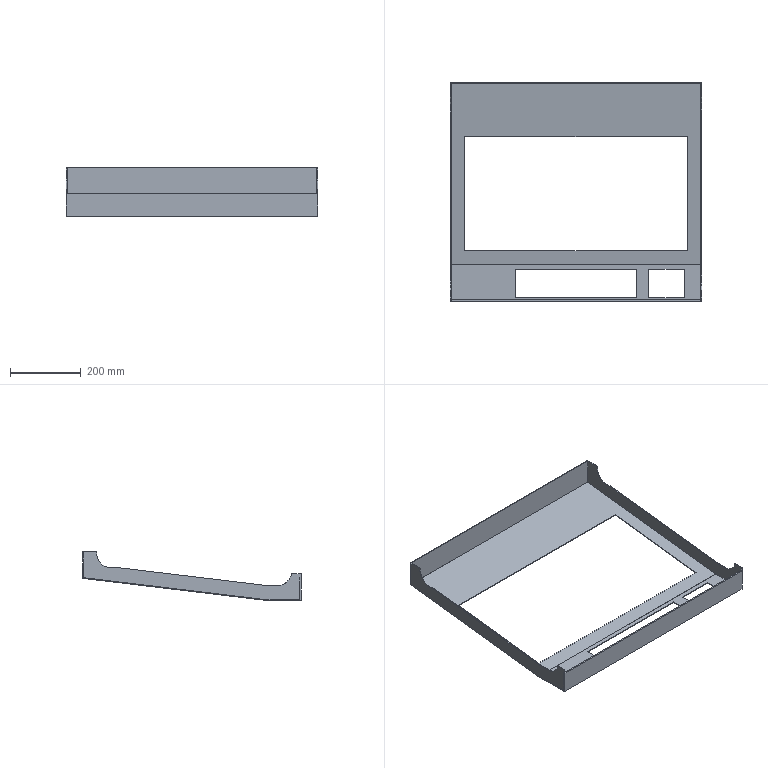Part | SolidWorks | features ICE 5, Cut 1, Extrusion 1 | 1 solid | 38 faces | box 710 x 618 x 137 mm | volume 789062 mm3 | plane 32 | cylinder 6 | commonest cylinder face diameters 80 x6
STEP:
#1=CARTESIAN_POINT('',(-708.,-79.693,30.051));
#2=VERTEX_POINT('',#1);
#3=CARTESIAN_POINT('',(-708.,-40.,75.));
#4=VERTEX_POINT('',#3);
#5=CARTESIAN_POINT('',(-708.,-79.693,70.051));
#6=DIRECTION('',(1.,0.,0.));
#7=DIRECTION('',(0.,0.,1.));
#8=AXIS2_PLACEMENT_3D('',#5,#6,#7);
#9=CIRCLE('',#8,40.);
#10=EDGE_CURVE('',#2,#4,#9,.T.);
#11=ORIENTED_EDGE('',*,*,#10,.F.);
#12=CARTESIAN_POINT('',(-706.,-79.693,30.051));
#13=VERTEX_POINT('',#12);
#14=CARTESIAN_POINT('',(-708.,-79.693,30.051));
#15=DIRECTION('',(1.,0.,0.));
#16=VECTOR('',#15,1000.);
#17=LINE('',#14,#16);
#18=EDGE_CURVE('',#2,#13,#17,.T.);
#19=ORIENTED_EDGE('',*,*,#18,.T.);
#20=CARTESIAN_POINT('',(-706.,-40.,75.));
#21=VERTEX_POINT('',#20);
#22=CARTESIAN_POINT('',(-706.,-79.693,70.051));
#23=DIRECTION('',(1.,0.,0.));
#24=DIRECTION('',(0.,0.,1.));
#25=AXIS2_PLACEMENT_3D('',#22,#23,#24);
#26=CIRCLE('',#25,40.);
#27=EDGE_CURVE('',#13,#21,#26,.T.);
#28=ORIENTED_EDGE('',*,*,#27,.T.);
#29=CARTESIAN_POINT('',(-708.,-40.,75.));
#30=DIRECTION('',(1.,0.,0.));
#31=VECTOR('',#30,1000.);
#32=LINE('',#29,#31);
#33=EDGE_CURVE('',#4,#21,#32,.T.);
#34=ORIENTED_EDGE('',*,*,#33,.F.);
#35=EDGE_LOOP('',(#11,#19,#28,#34));
#36=FACE_OUTER_BOUND('',#35,.T.);
#37=CARTESIAN_POINT('',(-708.,-79.693,70.051));
#38=DIRECTION('',(1.,0.,0.));
#39=DIRECTION('',(0.,0.,-1.));
#40=AXIS2_PLACEMENT_3D('',#37,#38,#39);
#41=CYLINDRICAL_SURFACE('',#40,40.);
#42=ADVANCED_FACE('',(#36),#41,.F.);
#43=CARTESIAN_POINT('',(-708.,-551.363,-20.439));
#44=VERTEX_POINT('',#43);
#45=CARTESIAN_POINT('',(-708.,-543.692,-19.697));
#46=VERTEX_POINT('',#45);
#47=CARTESIAN_POINT('',(-708.,-551.363,19.561));
#48=DIRECTION('',(1.,0.,0.));
#49=DIRECTION('',(0.,0.,1.));
#50=AXIS2_PLACEMENT_3D('',#47,#48,#49);
#51=CIRCLE('',#50,40.);
#52=EDGE_CURVE('',#44,#46,#51,.T.);
#53=ORIENTED_EDGE('',*,*,#52,.F.);
#54=CARTESIAN_POINT('',(-706.,-551.363,-20.439));
#55=VERTEX_POINT('',#54);
#56=CARTESIAN_POINT('',(-708.,-551.363,-20.439));
#57=DIRECTION('',(1.,0.,0.));
#58=VECTOR('',#57,1000.);
#59=LINE('',#56,#58);
#60=EDGE_CURVE('',#44,#55,#59,.T.);
#61=ORIENTED_EDGE('',*,*,#60,.T.);
#62=CARTESIAN_POINT('',(-706.,-543.692,-19.697));
#63=VERTEX_POINT('',#62);
#64=CARTESIAN_POINT('',(-706.,-551.363,19.561));
#65=DIRECTION('',(1.,0.,0.));
#66=DIRECTION('',(0.,0.,1.));
#67=AXIS2_PLACEMENT_3D('',#64,#65,#66);
#68=CIRCLE('',#67,40.);
#69=EDGE_CURVE('',#55,#63,#68,.T.);
#70=ORIENTED_EDGE('',*,*,#69,.T.);
#71=CARTESIAN_POINT('',(-708.,-543.692,-19.697));
#72=DIRECTION('',(1.,0.,0.));
#73=VECTOR('',#72,1000.);
#74=LINE('',#71,#73);
#75=EDGE_CURVE('',#46,#63,#74,.T.);
#76=ORIENTED_EDGE('',*,*,#75,.F.);
#77=EDGE_LOOP('',(#53,#61,#70,#76));
#78=FACE_OUTER_BOUND('',#77,.T.);
#79=CARTESIAN_POINT('',(-708.,-551.363,19.561));
#80=DIRECTION('',(1.,0.,0.));
#81=DIRECTION('',(0.,0.,-1.));
#82=AXIS2_PLACEMENT_3D('',#79,#80,#81);
#83=CYLINDRICAL_SURFACE('',#82,40.);
#84=ADVANCED_FACE('',(#78),#83,.F.);
#85=CARTESIAN_POINT('',(0.,-614.,1.));
#86=VERTEX_POINT('',#85);
#87=CARTESIAN_POINT('',(0.,-614.,-60.));
#88=VERTEX_POINT('',#87);
#89=CARTESIAN_POINT('',(0.,-614.,1.));
#90=DIRECTION('',(0.,0.,-1.));
#91=VECTOR('',#90,1000.);
#92=LINE('',#89,#91);
#93=EDGE_CURVE('',#86,#88,#92,.T.);
#94=ORIENTED_EDGE('',*,*,#93,.F.);
#95=CARTESIAN_POINT('',(0.,-618.,1.));
#96=VERTEX_POINT('',#95);
#97=CARTESIAN_POINT('',(0.,-618.,1.));
#98=DIRECTION('',(0.,1.,0.));
#99=VECTOR('',#98,1000.);
#100=LINE('',#97,#99);
#101=EDGE_CURVE('',#96,#86,#100,.T.);
#102=ORIENTED_EDGE('',*,*,#101,.F.);
#103=CARTESIAN_POINT('',(0.,-618.,13.));
#104=VERTEX_POINT('',#103);
#105=CARTESIAN_POINT('',(0.,-618.,13.));
#106=DIRECTION('',(0.,0.,-1.));
#107=VECTOR('',#106,1000.);
#108=LINE('',#105,#107);
#109=EDGE_CURVE('',#104,#96,#108,.T.);
#110=ORIENTED_EDGE('',*,*,#109,.F.);
#111=CARTESIAN_POINT('',(0.,-590.821,13.));
#112=VERTEX_POINT('',#111);
#113=CARTESIAN_POINT('',(0.,-618.,13.));
#114=DIRECTION('',(0.,-1.,0.));
#115=VECTOR('',#114,1000.);
#116=LINE('',#113,#115);
#117=EDGE_CURVE('',#112,#104,#116,.T.);
#118=ORIENTED_EDGE('',*,*,#117,.F.);
#119=CARTESIAN_POINT('',(0.,-543.692,-19.697));
#120=VERTEX_POINT('',#119);
#121=CARTESIAN_POINT('',(0.,-551.363,19.561));
#122=DIRECTION('',(-1.,0.,0.));
#123=DIRECTION('',(0.,0.,-1.));
#124=AXIS2_PLACEMENT_3D('',#121,#122,#123);
#125=CIRCLE('',#124,40.);
#126=EDGE_CURVE('',#120,#112,#125,.T.);
#127=ORIENTED_EDGE('',*,*,#126,.F.);
#128=CARTESIAN_POINT('',(0.,-515.,-19.697));
#129=VERTEX_POINT('',#128);
#130=CARTESIAN_POINT('',(0.,-515.,-19.697));
#131=DIRECTION('',(0.,-1.,0.));
#132=VECTOR('',#131,1000.);
#133=LINE('',#130,#132);
#134=EDGE_CURVE('',#129,#120,#133,.T.);
#135=ORIENTED_EDGE('',*,*,#134,.F.);
#136=CARTESIAN_POINT('',(0.,-90.171,31.448));
#137=VERTEX_POINT('',#136);
#138=CARTESIAN_POINT('',(0.,-90.171,31.448));
#139=DIRECTION('',(0.,-0.9928,-0.1195));
#140=VECTOR('',#139,1000.);
#141=LINE('',#138,#140);
#142=EDGE_CURVE('',#137,#129,#141,.T.);
#143=ORIENTED_EDGE('',*,*,#142,.F.);
#144=CARTESIAN_POINT('',(0.,-40.,75.));
#145=VERTEX_POINT('',#144);
#146=CARTESIAN_POINT('',(0.,-79.693,70.051));
#147=DIRECTION('',(-1.,0.,0.));
#148=DIRECTION('',(0.,0.,-1.));
#149=AXIS2_PLACEMENT_3D('',#146,#147,#148);
#150=CIRCLE('',#149,40.);
#151=EDGE_CURVE('',#145,#137,#150,.T.);
#152=ORIENTED_EDGE('',*,*,#151,.F.);
#153=CARTESIAN_POINT('',(0.,-2.,75.));
#154=VERTEX_POINT('',#153);
#155=CARTESIAN_POINT('',(0.,0.,75.));
#156=DIRECTION('',(0.,-1.,0.));
#157=VECTOR('',#156,1000.);
#158=LINE('',#155,#157);
#159=EDGE_CURVE('',#154,#145,#158,.T.);
#160=ORIENTED_EDGE('',*,*,#159,.F.);
#161=CARTESIAN_POINT('',(0.,-2.,1.774));
#162=VERTEX_POINT('',#161);
#163=CARTESIAN_POINT('',(0.,-2.,1.774));
#164=DIRECTION('',(0.,0.,1.));
#165=VECTOR('',#164,1000.);
#166=LINE('',#163,#165);
#167=EDGE_CURVE('',#162,#154,#166,.T.);
#168=ORIENTED_EDGE('',*,*,#167,.F.);
#169=CARTESIAN_POINT('',(0.,-515.12,-60.));
#170=VERTEX_POINT('',#169);
#171=CARTESIAN_POINT('',(0.,-515.12,-60.));
#172=DIRECTION('',(0.,0.9928,0.1195));
#173=VECTOR('',#172,1000.);
#174=LINE('',#171,#173);
#175=EDGE_CURVE('',#170,#162,#174,.T.);
#176=ORIENTED_EDGE('',*,*,#175,.F.);
#177=CARTESIAN_POINT('',(0.,-616.,-60.));
#178=DIRECTION('',(0.,1.,0.));
#179=VECTOR('',#178,1000.);
#180=LINE('',#177,#179);
#181=EDGE_CURVE('',#88,#170,#180,.T.);
#182=ORIENTED_EDGE('',*,*,#181,.F.);
#183=EDGE_LOOP('',(#94,#102,#110,#118,#127,#135,#143,#152,#160,#168,#176,#182));
#184=FACE_OUTER_BOUND('',#183,.T.);
#185=CARTESIAN_POINT('',(0.,-79.693,70.051));
#186=DIRECTION('',(1.,0.,0.));
#187=DIRECTION('',(0.,0.,-1.));
#188=AXIS2_PLACEMENT_3D('',#185,#186,#187);
#189=PLANE('',#188);
#190=ADVANCED_FACE('',(#184),#189,.F.);
#191=CARTESIAN_POINT('',(-147.,-528.,-60.));
#192=VERTEX_POINT('',#191);
#193=CARTESIAN_POINT('',(-47.,-528.,-60.));
#194=VERTEX_POINT('',#193);
#195=CARTESIAN_POINT('',(-147.,-528.,-60.));
#196=DIRECTION('',(1.,0.,0.));
#197=VECTOR('',#196,1000.);
#198=LINE('',#195,#197);
#199=EDGE_CURVE('',#192,#194,#198,.T.);
#200=ORIENTED_EDGE('',*,*,#199,.T.);
#201=CARTESIAN_POINT('',(-47.,-608.,-60.));
#202=VERTEX_POINT('',#201);
#203=CARTESIAN_POINT('',(-47.,-528.,-60.));
#204=DIRECTION('',(0.,-1.,0.));
#205=VECTOR('',#204,1000.);
#206=LINE('',#203,#205);
#207=EDGE_CURVE('',#194,#202,#206,.T.);
#208=ORIENTED_EDGE('',*,*,#207,.T.);
#209=CARTESIAN_POINT('',(-147.,-608.,-60.));
#210=VERTEX_POINT('',#209);
#211=CARTESIAN_POINT('',(-47.,-608.,-60.));
#212=DIRECTION('',(-1.,0.,0.));
#213=VECTOR('',#212,1000.);
#214=LINE('',#211,#213);
#215=EDGE_CURVE('',#202,#210,#214,.T.);
#216=ORIENTED_EDGE('',*,*,#215,.T.);
#217=CARTESIAN_POINT('',(-147.,-608.,-60.));
#218=DIRECTION('',(0.,1.,0.));
#219=VECTOR('',#218,1000.);
#220=LINE('',#217,#219);
#221=EDGE_CURVE('',#210,#192,#220,.T.);
#222=ORIENTED_EDGE('',*,*,#221,.T.);
#223=EDGE_LOOP('',(#200,#208,#216,#222));
#224=FACE_BOUND('',#223,.T.);
#225=CARTESIAN_POINT('',(-525.,-528.,-60.));
#226=VERTEX_POINT('',#225);
#227=CARTESIAN_POINT('',(-181.,-528.,-60.));
#228=VERTEX_POINT('',#227);
#229=CARTESIAN_POINT('',(-525.,-528.,-60.));
#230=DIRECTION('',(1.,0.,0.));
#231=VECTOR('',#230,1000.);
#232=LINE('',#229,#231);
#233=EDGE_CURVE('',#226,#228,#232,.T.);
#234=ORIENTED_EDGE('',*,*,#233,.T.);
#235=CARTESIAN_POINT('',(-181.,-608.,-60.));
#236=VERTEX_POINT('',#235);
#237=CARTESIAN_POINT('',(-181.,-528.,-60.));
#238=DIRECTION('',(0.,-1.,0.));
#239=VECTOR('',#238,1000.);
#240=LINE('',#237,#239);
#241=EDGE_CURVE('',#228,#236,#240,.T.);
#242=ORIENTED_EDGE('',*,*,#241,.T.);
#243=CARTESIAN_POINT('',(-525.,-608.,-60.));
#244=VERTEX_POINT('',#243);
#245=CARTESIAN_POINT('',(-181.,-608.,-60.));
#246=DIRECTION('',(-1.,0.,0.));
#247=VECTOR('',#246,1000.);
#248=LINE('',#245,#247);
#249=EDGE_CURVE('',#236,#244,#248,.T.);
#250=ORIENTED_EDGE('',*,*,#249,.T.);
#251=CARTESIAN_POINT('',(-525.,-608.,-60.));
#252=DIRECTION('',(0.,1.,0.));
#253=VECTOR('',#252,1000.);
#254=LINE('',#251,#253);
#255=EDGE_CURVE('',#244,#226,#254,.T.);
#256=ORIENTED_EDGE('',*,*,#255,.T.);
#257=EDGE_LOOP('',(#234,#242,#250,#256));
#258=FACE_BOUND('',#257,.T.);
#259=CARTESIAN_POINT('',(-706.,-614.,-60.));
#260=VERTEX_POINT('',#259);
#261=CARTESIAN_POINT('',(-706.,-614.,-60.));
#262=DIRECTION('',(-1.,0.,0.));
#263=VECTOR('',#262,1000.);
#264=LINE('',#261,#263);
#265=EDGE_CURVE('',#88,#260,#264,.T.);
#266=ORIENTED_EDGE('',*,*,#265,.F.);
#267=ORIENTED_EDGE('',*,*,#181,.T.);
#268=CARTESIAN_POINT('',(-706.,-515.12,-60.));
#269=VERTEX_POINT('',#268);
#270=CARTESIAN_POINT('',(-706.,-515.12,-60.));
#271=DIRECTION('',(1.,0.,0.));
#272=VECTOR('',#271,1000.);
#273=LINE('',#270,#272);
#274=EDGE_CURVE('',#269,#170,#273,.T.);
#275=ORIENTED_EDGE('',*,*,#274,.F.);
#276=CARTESIAN_POINT('',(-706.,-616.,-60.));
#277=DIRECTION('',(0.,1.,0.));
#278=VECTOR('',#277,1000.);
#279=LINE('',#276,#278);
#280=EDGE_CURVE('',#260,#269,#279,.T.);
#281=ORIENTED_EDGE('',*,*,#280,.F.);
#282=EDGE_LOOP('',(#266,#267,#275,#281));
#283=FACE_OUTER_BOUND('',#282,.T.);
#284=CARTESIAN_POINT('',(-706.,-616.,-60.));
#285=DIRECTION('',(0.,0.,-1.));
#286=DIRECTION('',(-1.,0.,0.));
#287=AXIS2_PLACEMENT_3D('',#284,#285,#286);
#288=PLANE('',#287);
#289=ADVANCED_FACE('',(#224,#258,#283),#288,.F.);
#290=CARTESIAN_POINT('',(-706.,-614.,1.));
#291=VERTEX_POINT('',#290);
#292=CARTESIAN_POINT('',(-706.,-614.,1.));
#293=DIRECTION('',(0.,0.,-1.));
#294=VECTOR('',#293,1000.);
#295=LINE('',#292,#294);
#296=EDGE_CURVE('',#291,#260,#295,.T.);
#297=ORIENTED_EDGE('',*,*,#296,.T.);
#298=ORIENTED_EDGE('',*,*,#280,.T.);
#299=CARTESIAN_POINT('',(-706.,-2.,1.774));
#300=VERTEX_POINT('',#299);
#301=CARTESIAN_POINT('',(-706.,-515.12,-60.));
#302=DIRECTION('',(0.,0.9928,0.1195));
#303=VECTOR('',#302,1000.);
#304=LINE('',#301,#303);
#305=EDGE_CURVE('',#269,#300,#304,.T.);
#306=ORIENTED_EDGE('',*,*,#305,.T.);
#307=CARTESIAN_POINT('',(-706.,-2.,75.));
#308=VERTEX_POINT('',#307);
#309=CARTESIAN_POINT('',(-706.,-2.,1.774));
#310=DIRECTION('',(0.,0.,1.));
#311=VECTOR('',#310,1000.);
#312=LINE('',#309,#311);
#313=EDGE_CURVE('',#300,#308,#312,.T.);
#314=ORIENTED_EDGE('',*,*,#313,.T.);
#315=CARTESIAN_POINT('',(-706.,-40.,75.));
#316=DIRECTION('',(0.,1.,0.));
#317=VECTOR('',#316,1000.);
#318=LINE('',#315,#317);
#319=EDGE_CURVE('',#21,#308,#318,.T.);
#320=ORIENTED_EDGE('',*,*,#319,.F.);
#321=ORIENTED_EDGE('',*,*,#27,.F.);
#322=CARTESIAN_POINT('',(-706.,-90.171,31.448));
#323=VERTEX_POINT('',#322);
#324=CARTESIAN_POINT('',(-706.,-79.693,70.051));
#325=DIRECTION('',(1.,0.,0.));
#326=DIRECTION('',(0.,0.,1.));
#327=AXIS2_PLACEMENT_3D('',#324,#325,#326);
#328=CIRCLE('',#327,40.);
#329=EDGE_CURVE('',#323,#13,#328,.T.);
#330=ORIENTED_EDGE('',*,*,#329,.F.);
#331=CARTESIAN_POINT('',(-706.,-515.,-19.697));
#332=VERTEX_POINT('',#331);
#333=CARTESIAN_POINT('',(-706.,-515.,-19.697));
#334=DIRECTION('',(0.,0.9928,0.1195));
#335=VECTOR('',#334,1000.);
#336=LINE('',#333,#335);
#337=EDGE_CURVE('',#332,#323,#336,.T.);
#338=ORIENTED_EDGE('',*,*,#337,.F.);
#339=CARTESIAN_POINT('',(-706.,-543.692,-19.697));
#340=DIRECTION('',(0.,1.,0.));
#341=VECTOR('',#340,1000.);
#342=LINE('',#339,#341);
#343=EDGE_CURVE('',#63,#332,#342,.T.);
#344=ORIENTED_EDGE('',*,*,#343,.F.);
#345=ORIENTED_EDGE('',*,*,#69,.F.);
#346=CARTESIAN_POINT('',(-706.,-590.821,13.));
#347=VERTEX_POINT('',#346);
#348=CARTESIAN_POINT('',(-706.,-551.363,19.561));
#349=DIRECTION('',(1.,0.,0.));
#350=DIRECTION('',(0.,0.,1.));
#351=AXIS2_PLACEMENT_3D('',#348,#349,#350);
#352=CIRCLE('',#351,40.);
#353=EDGE_CURVE('',#347,#55,#352,.T.);
#354=ORIENTED_EDGE('',*,*,#353,.F.);
#355=CARTESIAN_POINT('',(-706.,-618.,13.));
#356=VERTEX_POINT('',#355);
#357=CARTESIAN_POINT('',(-706.,-618.,13.));
#358=DIRECTION('',(0.,1.,0.));
#359=VECTOR('',#358,1000.);
#360=LINE('',#357,#359);
#361=EDGE_CURVE('',#356,#347,#360,.T.);
#362=ORIENTED_EDGE('',*,*,#361,.F.);
#363=CARTESIAN_POINT('',(-706.,-618.,1.));
#364=VERTEX_POINT('',#363);
#365=CARTESIAN_POINT('',(-706.,-618.,-62.));
#366=DIRECTION('',(0.,0.,1.));
#367=VECTOR('',#366,1000.);
#368=LINE('',#365,#367);
#369=EDGE_CURVE('',#364,#356,#368,.T.);
#370=ORIENTED_EDGE('',*,*,#369,.F.);
#371=CARTESIAN_POINT('',(-706.,-618.,1.));
#372=DIRECTION('',(0.,-1.,0.));
#373=VECTOR('',#372,1000.);
#374=LINE('',#371,#373);
#375=EDGE_CURVE('',#291,#364,#374,.T.);
#376=ORIENTED_EDGE('',*,*,#375,.F.);
#377=EDGE_LOOP('',(#297,#298,#306,#314,#320,#321,#330,#338,#344,#345,#354,#362,#370,#376));
#378=FACE_OUTER_BOUND('',#377,.T.);
#379=CARTESIAN_POINT('',(-706.,-551.363,19.561));
#380=DIRECTION('',(-1.,0.,0.));
#381=DIRECTION('',(0.,0.,1.));
#382=AXIS2_PLACEMENT_3D('',#379,#380,#381);
#383=PLANE('',#382);
#384=ADVANCED_FACE('',(#378),#383,.F.);
#385=CARTESIAN_POINT('',(-667.,-152.,-18.299));
#386=VERTEX_POINT('',#385);
#387=CARTESIAN_POINT('',(-39.,-152.,-18.299));
#388=VERTEX_POINT('',#387);
#389=CARTESIAN_POINT('',(-39.,-152.,-18.299));
#390=DIRECTION('',(1.,0.,0.));
#391=VECTOR('',#390,1000.);
#392=LINE('',#389,#391);
#393=EDGE_CURVE('',#386,#388,#392,.T.);
#394=ORIENTED_EDGE('',*,*,#393,.F.);
#395=CARTESIAN_POINT('',(-667.,-475.,-57.184));
#396=VERTEX_POINT('',#395);
#397=CARTESIAN_POINT('',(-667.,-140.928,-16.966));
#398=DIRECTION('',(0.,0.9928,0.1195));
#399=VECTOR('',#398,1000.);
#400=LINE('',#397,#399);
#401=EDGE_CURVE('',#396,#386,#400,.T.);
#402=ORIENTED_EDGE('',*,*,#401,.F.);
#403=CARTESIAN_POINT('',(-39.,-475.,-57.184));
#404=VERTEX_POINT('',#403);
#405=CARTESIAN_POINT('',(-39.,-475.,-57.184));
#406=DIRECTION('',(-1.,0.,0.));
#407=VECTOR('',#406,1000.);
#408=LINE('',#405,#407);
#409=EDGE_CURVE('',#404,#396,#408,.T.);
#410=ORIENTED_EDGE('',*,*,#409,.F.);
#411=CARTESIAN_POINT('',(-39.,-140.928,-16.966));
#412=DIRECTION('',(0.,-0.9928,-0.1195));
#413=VECTOR('',#412,1000.);
#414=LINE('',#411,#413);
#415=EDGE_CURVE('',#388,#404,#414,.T.);
#416=ORIENTED_EDGE('',*,*,#415,.F.);
#417=EDGE_LOOP('',(#394,#402,#410,#416));
#418=FACE_BOUND('',#417,.T.);
#419=CARTESIAN_POINT('',(2.,-515.,-62.));
#420=VERTEX_POINT('',#419);
#421=CARTESIAN_POINT('',(-708.,-515.,-62.));
#422=VERTEX_POINT('',#421);
#423=CARTESIAN_POINT('',(2.,-515.,-62.));
#424=DIRECTION('',(-1.,0.,0.));
#425=VECTOR('',#424,1000.);
#426=LINE('',#423,#425);
#427=EDGE_CURVE('',#420,#422,#426,.T.);
#428=ORIENTED_EDGE('',*,*,#427,.T.);
#429=CARTESIAN_POINT('',(-708.,0.,0.));
#430=VERTEX_POINT('',#429);
#431=CARTESIAN_POINT('',(-708.,0.,0.));
#432=DIRECTION('',(0.,-0.9928,-0.1195));
#433=VECTOR('',#432,1000.);
#434=LINE('',#431,#433);
#435=EDGE_CURVE('',#430,#422,#434,.T.);
#436=ORIENTED_EDGE('',*,*,#435,.F.);
#437=CARTESIAN_POINT('',(2.,0.,0.));
#438=VERTEX_POINT('',#437);
#439=CARTESIAN_POINT('',(2.,0.,0.));
#440=DIRECTION('',(-1.,0.,0.));
#441=VECTOR('',#440,1000.);
#442=LINE('',#439,#441);
#443=EDGE_CURVE('',#438,#430,#442,.T.);
#444=ORIENTED_EDGE('',*,*,#443,.F.);
#445=CARTESIAN_POINT('',(2.,-515.,-62.));
#446=DIRECTION('',(0.,0.9928,0.1195));
#447=VECTOR('',#446,1000.);
#448=LINE('',#445,#447);
#449=EDGE_CURVE('',#420,#438,#448,.T.);
#450=ORIENTED_EDGE('',*,*,#449,.F.);
#451=EDGE_LOOP('',(#428,#436,#444,#450));
#452=FACE_OUTER_BOUND('',#451,.T.);
#453=CARTESIAN_POINT('',(2.,-515.,-62.));
#454=DIRECTION('',(0.,-0.1195,0.9928));
#455=DIRECTION('',(0.,-0.9928,-0.1195));
#456=AXIS2_PLACEMENT_3D('',#453,#454,#455);
#457=PLANE('',#456);
#458=ADVANCED_FACE('',(#418,#452),#457,.F.);
#459=ORIENTED_EDGE('',*,*,#443,.T.);
#460=CARTESIAN_POINT('',(-708.,0.,75.));
#461=VERTEX_POINT('',#460);
#462=CARTESIAN_POINT('',(-708.,0.,75.));
#463=DIRECTION('',(0.,0.,-1.));
#464=VECTOR('',#463,1000.);
#465=LINE('',#462,#464);
#466=EDGE_CURVE('',#461,#430,#465,.T.);
#467=ORIENTED_EDGE('',*,*,#466,.F.);
#468=CARTESIAN_POINT('',(2.,0.,75.));
#469=VERTEX_POINT('',#468);
#470=CARTESIAN_POINT('',(2.,0.,75.));
#471=DIRECTION('',(-1.,0.,0.));
#472=VECTOR('',#471,1000.);
#473=LINE('',#470,#472);
#474=EDGE_CURVE('',#469,#461,#473,.T.);
#475=ORIENTED_EDGE('',*,*,#474,.F.);
#476=CARTESIAN_POINT('',(2.,0.,0.));
#477=DIRECTION('',(0.,0.,1.));
#478=VECTOR('',#477,1000.);
#479=LINE('',#476,#478);
#480=EDGE_CURVE('',#438,#469,#479,.T.);
#481=ORIENTED_EDGE('',*,*,#480,.F.);
#482=EDGE_LOOP('',(#459,#467,#475,#481));
#483=FACE_OUTER_BOUND('',#482,.T.);
#484=CARTESIAN_POINT('',(2.,0.,0.));
#485=DIRECTION('',(0.,-1.,0.));
#486=DIRECTION('',(0.,0.,-1.));
#487=AXIS2_PLACEMENT_3D('',#484,#485,#486);
#488=PLANE('',#487);
#489=ADVANCED_FACE('',(#483),#488,.F.);
#490=ORIENTED_EDGE('',*,*,#474,.T.);
#491=CARTESIAN_POINT('',(-708.,-40.,75.));
#492=DIRECTION('',(0.,1.,0.));
#493=VECTOR('',#492,1000.);
#494=LINE('',#491,#493);
#495=EDGE_CURVE('',#4,#461,#494,.T.);
#496=ORIENTED_EDGE('',*,*,#495,.F.);
#497=ORIENTED_EDGE('',*,*,#33,.T.);
#498=ORIENTED_EDGE('',*,*,#319,.T.);
#499=CARTESIAN_POINT('',(-706.,-2.,75.));
#500=DIRECTION('',(1.,0.,0.));
#501=VECTOR('',#500,1000.);
#502=LINE('',#499,#501);
#503=EDGE_CURVE('',#308,#154,#502,.T.);
#504=ORIENTED_EDGE('',*,*,#503,.T.);
#505=ORIENTED_EDGE('',*,*,#159,.T.);
#506=CARTESIAN_POINT('',(2.,-40.,75.));
#507=VERTEX_POINT('',#506);
#508=CARTESIAN_POINT('',(2.,-40.,75.));
#509=DIRECTION('',(-1.,0.,0.));
#510=VECTOR('',#509,1000.);
#511=LINE('',#508,#510);
#512=EDGE_CURVE('',#507,#145,#511,.T.);
#513=ORIENTED_EDGE('',*,*,#512,.F.);
#514=CARTESIAN_POINT('',(2.,0.,75.));
#515=DIRECTION('',(0.,-1.,0.));
#516=VECTOR('',#515,1000.);
#517=LINE('',#514,#516);
#518=EDGE_CURVE('',#469,#507,#517,.T.);
#519=ORIENTED_EDGE('',*,*,#518,.F.);
#520=EDGE_LOOP('',(#490,#496,#497,#498,#504,#505,#513,#519));
#521=FACE_OUTER_BOUND('',#520,.T.);
#522=CARTESIAN_POINT('',(2.,0.,75.));
#523=DIRECTION('',(0.,0.,-1.));
#524=DIRECTION('',(-1.,0.,0.));
#525=AXIS2_PLACEMENT_3D('',#522,#523,#524);
#526=PLANE('',#525);
#527=ADVANCED_FACE('',(#521),#526,.F.);
#528=ORIENTED_EDGE('',*,*,#151,.T.);
#529=CARTESIAN_POINT('',(2.,-90.171,31.448));
#530=VERTEX_POINT('',#529);
#531=CARTESIAN_POINT('',(2.,-90.171,31.448));
#532=DIRECTION('',(-1.,0.,0.));
#533=VECTOR('',#532,1000.);
#534=LINE('',#531,#533);
#535=EDGE_CURVE('',#530,#137,#534,.T.);
#536=ORIENTED_EDGE('',*,*,#535,.F.);
#537=CARTESIAN_POINT('',(2.,-79.693,70.051));
#538=DIRECTION('',(-1.,0.,0.));
#539=DIRECTION('',(0.,0.,-1.));
#540=AXIS2_PLACEMENT_3D('',#537,#538,#539);
#541=CIRCLE('',#540,40.);
#542=EDGE_CURVE('',#507,#530,#541,.T.);
#543=ORIENTED_EDGE('',*,*,#542,.F.);
#544=ORIENTED_EDGE('',*,*,#512,.T.);
#545=EDGE_LOOP('',(#528,#536,#543,#544));
#546=FACE_OUTER_BOUND('',#545,.T.);
#547=CARTESIAN_POINT('',(2.,-79.693,70.051));
#548=DIRECTION('',(-1.,0.,0.));
#549=DIRECTION('',(0.,0.,1.));
#550=AXIS2_PLACEMENT_3D('',#547,#548,#549);
#551=CYLINDRICAL_SURFACE('',#550,40.);
#552=ADVANCED_FACE('',(#546),#551,.F.);
#553=ORIENTED_EDGE('',*,*,#142,.T.);
#554=CARTESIAN_POINT('',(2.,-515.,-19.697));
#555=VERTEX_POINT('',#554);
#556=CARTESIAN_POINT('',(2.,-515.,-19.697));
#557=DIRECTION('',(-1.,0.,0.));
#558=VECTOR('',#557,1000.);
#559=LINE('',#556,#558);
#560=EDGE_CURVE('',#555,#129,#559,.T.);
#561=ORIENTED_EDGE('',*,*,#560,.F.);
#562=CARTESIAN_POINT('',(2.,-90.171,31.448));
#563=DIRECTION('',(0.,-0.9928,-0.1195));
#564=VECTOR('',#563,1000.);
#565=LINE('',#562,#564);
#566=EDGE_CURVE('',#530,#555,#565,.T.);
#567=ORIENTED_EDGE('',*,*,#566,.F.);
#568=ORIENTED_EDGE('',*,*,#535,.T.);
#569=EDGE_LOOP('',(#553,#561,#567,#568));
#570=FACE_OUTER_BOUND('',#569,.T.);
#571=CARTESIAN_POINT('',(2.,-90.171,31.448));
#572=DIRECTION('',(0.,0.1195,-0.9928));
#573=DIRECTION('',(0.,0.9928,0.1195));
#574=AXIS2_PLACEMENT_3D('',#571,#572,#573);
#575=PLANE('',#574);
#576=ADVANCED_FACE('',(#570),#575,.F.);
#577=ORIENTED_EDGE('',*,*,#134,.T.);
#578=CARTESIAN_POINT('',(2.,-543.692,-19.697));
#579=VERTEX_POINT('',#578);
#580=CARTESIAN_POINT('',(2.,-543.692,-19.697));
#581=DIRECTION('',(-1.,0.,0.));
#582=VECTOR('',#581,1000.);
#583=LINE('',#580,#582);
#584=EDGE_CURVE('',#579,#120,#583,.T.);
#585=ORIENTED_EDGE('',*,*,#584,.F.);
#586=CARTESIAN_POINT('',(2.,-515.,-19.697));
#587=DIRECTION('',(0.,-1.,0.));
#588=VECTOR('',#587,1000.);
#589=LINE('',#586,#588);
#590=EDGE_CURVE('',#555,#579,#589,.T.);
#591=ORIENTED_EDGE('',*,*,#590,.F.);
#592=ORIENTED_EDGE('',*,*,#560,.T.);
#593=EDGE_LOOP('',(#577,#585,#591,#592));
#594=FACE_OUTER_BOUND('',#593,.T.);
#595=CARTESIAN_POINT('',(2.,-515.,-19.697));
#596=DIRECTION('',(0.,0.,-1.));
#597=DIRECTION('',(-1.,0.,0.));
#598=AXIS2_PLACEMENT_3D('',#595,#596,#597);
#599=PLANE('',#598);
#600=ADVANCED_FACE('',(#594),#599,.F.);
#601=ORIENTED_EDGE('',*,*,#126,.T.);
#602=CARTESIAN_POINT('',(2.,-590.821,13.));
#603=VERTEX_POINT('',#602);
#604=CARTESIAN_POINT('',(2.,-590.821,13.));
#605=DIRECTION('',(-1.,0.,0.));
#606=VECTOR('',#605,1000.);
#607=LINE('',#604,#606);
#608=EDGE_CURVE('',#603,#112,#607,.T.);
#609=ORIENTED_EDGE('',*,*,#608,.F.);
#610=CARTESIAN_POINT('',(2.,-551.363,19.561));
#611=DIRECTION('',(-1.,0.,0.));
#612=DIRECTION('',(0.,0.,-1.));
#613=AXIS2_PLACEMENT_3D('',#610,#611,#612);
#614=CIRCLE('',#613,40.);
#615=EDGE_CURVE('',#579,#603,#614,.T.);
#616=ORIENTED_EDGE('',*,*,#615,.F.);
#617=ORIENTED_EDGE('',*,*,#584,.T.);
#618=EDGE_LOOP('',(#601,#609,#616,#617));
#619=FACE_OUTER_BOUND('',#618,.T.);
#620=CARTESIAN_POINT('',(2.,-551.363,19.561));
#621=DIRECTION('',(-1.,0.,0.));
#622=DIRECTION('',(0.,0.,1.));
#623=AXIS2_PLACEMENT_3D('',#620,#621,#622);
#624=CYLINDRICAL_SURFACE('',#623,40.);
#625=ADVANCED_FACE('',(#619),#624,.F.);
#626=ORIENTED_EDGE('',*,*,#117,.T.);
#627=CARTESIAN_POINT('',(2.,-618.,13.));
#628=VERTEX_POINT('',#627);
#629=CARTESIAN_POINT('',(2.,-618.,13.));
#630=DIRECTION('',(-1.,0.,0.));
#631=VECTOR('',#630,1000.);
#632=LINE('',#629,#631);
#633=EDGE_CURVE('',#628,#104,#632,.T.);
#634=ORIENTED_EDGE('',*,*,#633,.F.);
#635=CARTESIAN_POINT('',(2.,-618.,13.));
#636=DIRECTION('',(0.,-1.,0.));
#637=VECTOR('',#636,1000.);
#638=LINE('',#635,#637);
#639=EDGE_CURVE('',#603,#628,#638,.T.);
#640=ORIENTED_EDGE('',*,*,#639,.F.);
#641=ORIENTED_EDGE('',*,*,#608,.T.);
#642=EDGE_LOOP('',(#626,#634,#640,#641));
#643=FACE_OUTER_BOUND('',#642,.T.);
#644=CARTESIAN_POINT('',(2.,-618.,13.));
#645=DIRECTION('',(0.,0.,-1.));
#646=DIRECTION('',(-1.,0.,0.));
#647=AXIS2_PLACEMENT_3D('',#644,#645,#646);
#648=PLANE('',#647);
#649=ADVANCED_FACE('',(#643),#648,.F.);
#650=ORIENTED_EDGE('',*,*,#109,.T.);
#651=CARTESIAN_POINT('',(-706.,-618.,1.));
#652=DIRECTION('',(1.,0.,0.));
#653=VECTOR('',#652,1000.);
#654=LINE('',#651,#653);
#655=EDGE_CURVE('',#364,#96,#654,.T.);
#656=ORIENTED_EDGE('',*,*,#655,.F.);
#657=ORIENTED_EDGE('',*,*,#369,.T.);
#658=CARTESIAN_POINT('',(-708.,-618.,13.));
#659=VERTEX_POINT('',#658);
#660=CARTESIAN_POINT('',(-708.,-618.,13.));
#661=DIRECTION('',(1.,0.,0.));
#662=VECTOR('',#661,1000.);
#663=LINE('',#660,#662);
#664=EDGE_CURVE('',#659,#356,#663,.T.);
#665=ORIENTED_EDGE('',*,*,#664,.F.);
#666=CARTESIAN_POINT('',(-708.,-618.,-62.));
#667=VERTEX_POINT('',#666);
#668=CARTESIAN_POINT('',(-708.,-618.,-62.));
#669=DIRECTION('',(0.,0.,1.));
#670=VECTOR('',#669,1000.);
#671=LINE('',#668,#670);
#672=EDGE_CURVE('',#667,#659,#671,.T.);
#673=ORIENTED_EDGE('',*,*,#672,.F.);
#674=CARTESIAN_POINT('',(2.,-618.,-62.));
#675=VERTEX_POINT('',#674);
#676=CARTESIAN_POINT('',(2.,-618.,-62.));
#677=DIRECTION('',(-1.,0.,0.));
#678=VECTOR('',#677,1000.);
#679=LINE('',#676,#678);
#680=EDGE_CURVE('',#675,#667,#679,.T.);
#681=ORIENTED_EDGE('',*,*,#680,.F.);
#682=CARTESIAN_POINT('',(2.,-618.,13.));
#683=DIRECTION('',(0.,0.,-1.));
#684=VECTOR('',#683,1000.);
#685=LINE('',#682,#684);
#686=EDGE_CURVE('',#628,#675,#685,.T.);
#687=ORIENTED_EDGE('',*,*,#686,.F.);
#688=ORIENTED_EDGE('',*,*,#633,.T.);
#689=EDGE_LOOP('',(#650,#656,#657,#665,#673,#681,#687,#688));
#690=FACE_OUTER_BOUND('',#689,.T.);
#691=CARTESIAN_POINT('',(2.,-618.,13.));
#692=DIRECTION('',(0.,1.,0.));
#693=DIRECTION('',(0.,0.,1.));
#694=AXIS2_PLACEMENT_3D('',#691,#692,#693);
#695=PLANE('',#694);
#696=ADVANCED_FACE('',(#690),#695,.F.);
#697=CARTESIAN_POINT('',(-181.,-608.,-62.));
#698=VERTEX_POINT('',#697);
#699=CARTESIAN_POINT('',(-525.,-608.,-62.));
#700=VERTEX_POINT('',#699);
#701=CARTESIAN_POINT('',(-181.,-608.,-62.));
#702=DIRECTION('',(-1.,0.,0.));
#703=VECTOR('',#702,1000.);
#704=LINE('',#701,#703);
#705=EDGE_CURVE('',#698,#700,#704,.T.);
#706=ORIENTED_EDGE('',*,*,#705,.F.);
#707=CARTESIAN_POINT('',(-181.,-528.,-62.));
#708=VERTEX_POINT('',#707);
#709=CARTESIAN_POINT('',(-181.,-528.,-62.));
#710=DIRECTION('',(0.,-1.,0.));
#711=VECTOR('',#710,1000.);
#712=LINE('',#709,#711);
#713=EDGE_CURVE('',#708,#698,#712,.T.);
#714=ORIENTED_EDGE('',*,*,#713,.F.);
#715=CARTESIAN_POINT('',(-525.,-528.,-62.));
#716=VERTEX_POINT('',#715);
#717=CARTESIAN_POINT('',(-525.,-528.,-62.));
#718=DIRECTION('',(1.,0.,0.));
#719=VECTOR('',#718,1000.);
#720=LINE('',#717,#719);
#721=EDGE_CURVE('',#716,#708,#720,.T.);
#722=ORIENTED_EDGE('',*,*,#721,.F.);
#723=CARTESIAN_POINT('',(-525.,-608.,-62.));
#724=DIRECTION('',(0.,1.,0.));
#725=VECTOR('',#724,1000.);
#726=LINE('',#723,#725);
#727=EDGE_CURVE('',#700,#716,#726,.T.);
#728=ORIENTED_EDGE('',*,*,#727,.F.);
#729=EDGE_LOOP('',(#706,#714,#722,#728));
#730=FACE_BOUND('',#729,.T.);
#731=CARTESIAN_POINT('',(-47.,-608.,-62.));
#732=VERTEX_POINT('',#731);
#733=CARTESIAN_POINT('',(-147.,-608.,-62.));
#734=VERTEX_POINT('',#733);
#735=CARTESIAN_POINT('',(-47.,-608.,-62.));
#736=DIRECTION('',(-1.,0.,0.));
#737=VECTOR('',#736,1000.);
#738=LINE('',#735,#737);
#739=EDGE_CURVE('',#732,#734,#738,.T.);
#740=ORIENTED_EDGE('',*,*,#739,.F.);
#741=CARTESIAN_POINT('',(-47.,-528.,-62.));
#742=VERTEX_POINT('',#741);
#743=CARTESIAN_POINT('',(-47.,-528.,-62.));
#744=DIRECTION('',(0.,-1.,0.));
#745=VECTOR('',#744,1000.);
#746=LINE('',#743,#745);
#747=EDGE_CURVE('',#742,#732,#746,.T.);
#748=ORIENTED_EDGE('',*,*,#747,.F.);
#749=CARTESIAN_POINT('',(-147.,-528.,-62.));
#750=VERTEX_POINT('',#749);
#751=CARTESIAN_POINT('',(-147.,-528.,-62.));
#752=DIRECTION('',(1.,0.,0.));
#753=VECTOR('',#752,1000.);
#754=LINE('',#751,#753);
#755=EDGE_CURVE('',#750,#742,#754,.T.);
#756=ORIENTED_EDGE('',*,*,#755,.F.);
#757=CARTESIAN_POINT('',(-147.,-608.,-62.));
#758=DIRECTION('',(0.,1.,0.));
#759=VECTOR('',#758,1000.);
#760=LINE('',#757,#759);
#761=EDGE_CURVE('',#734,#750,#760,.T.);
#762=ORIENTED_EDGE('',*,*,#761,.F.);
#763=EDGE_LOOP('',(#740,#748,#756,#762));
#764=FACE_BOUND('',#763,.T.);
#765=ORIENTED_EDGE('',*,*,#680,.T.);
#766=CARTESIAN_POINT('',(-708.,-515.,-62.));
#767=DIRECTION('',(0.,-1.,0.));
#768=VECTOR('',#767,1000.);
#769=LINE('',#766,#768);
#770=EDGE_CURVE('',#422,#667,#769,.T.);
#771=ORIENTED_EDGE('',*,*,#770,.F.);
#772=ORIENTED_EDGE('',*,*,#427,.F.);
#773=CARTESIAN_POINT('',(2.,-618.,-62.));
#774=DIRECTION('',(0.,1.,0.));
#775=VECTOR('',#774,1000.);
#776=LINE('',#773,#775);
#777=EDGE_CURVE('',#675,#420,#776,.T.);
#778=ORIENTED_EDGE('',*,*,#777,.F.);
#779=EDGE_LOOP('',(#765,#771,#772,#778));
#780=FACE_OUTER_BOUND('',#779,.T.);
#781=CARTESIAN_POINT('',(2.,-618.,-62.));
#782=DIRECTION('',(0.,0.,1.));
#783=DIRECTION('',(1.,0.,0.));
#784=AXIS2_PLACEMENT_3D('',#781,#782,#783);
#785=PLANE('',#784);
#786=ADVANCED_FACE('',(#730,#764,#780),#785,.F.);
#787=ORIENTED_EDGE('',*,*,#449,.T.);
#788=ORIENTED_EDGE('',*,*,#480,.T.);
#789=ORIENTED_EDGE('',*,*,#518,.T.);
#790=ORIENTED_EDGE('',*,*,#542,.T.);
#791=ORIENTED_EDGE('',*,*,#566,.T.);
#792=ORIENTED_EDGE('',*,*,#590,.T.);
#793=ORIENTED_EDGE('',*,*,#615,.T.);
#794=ORIENTED_EDGE('',*,*,#639,.T.);
#795=ORIENTED_EDGE('',*,*,#686,.T.);
#796=ORIENTED_EDGE('',*,*,#777,.T.);
#797=EDGE_LOOP('',(#787,#788,#789,#790,#791,#792,#793,#794,#795,#796));
#798=FACE_OUTER_BOUND('',#797,.T.);
#799=CARTESIAN_POINT('',(2.,-79.693,70.051));
#800=DIRECTION('',(1.,0.,0.));
#801=DIRECTION('',(0.,0.,-1.));
#802=AXIS2_PLACEMENT_3D('',#799,#800,#801);
#803=PLANE('',#802);
#804=ADVANCED_FACE('',(#798),#803,.T.);
#805=CARTESIAN_POINT('',(-667.,-475.,-55.17));
#806=VERTEX_POINT('',#805);
#807=CARTESIAN_POINT('',(-39.,-475.,-55.17));
#808=VERTEX_POINT('',#807);
#809=CARTESIAN_POINT('',(-39.,-475.,-55.17));
#810=DIRECTION('',(1.,0.,0.));
#811=VECTOR('',#810,1000.);
#812=LINE('',#809,#811);
#813=EDGE_CURVE('',#806,#808,#812,.T.);
#814=ORIENTED_EDGE('',*,*,#813,.F.);
#815=CARTESIAN_POINT('',(-667.,-152.,-16.285));
#816=VERTEX_POINT('',#815);
#817=CARTESIAN_POINT('',(-667.,-141.167,-14.98));
#818=DIRECTION('',(0.,-0.9928,-0.1195));
#819=VECTOR('',#818,1000.);
#820=LINE('',#817,#819);
#821=EDGE_CURVE('',#816,#806,#820,.T.);
#822=ORIENTED_EDGE('',*,*,#821,.F.);
#823=CARTESIAN_POINT('',(-39.,-152.,-16.285));
#824=VERTEX_POINT('',#823);
#825=CARTESIAN_POINT('',(-39.,-152.,-16.285));
#826=DIRECTION('',(-1.,0.,0.));
#827=VECTOR('',#826,1000.);
#828=LINE('',#825,#827);
#829=EDGE_CURVE('',#824,#816,#828,.T.);
#830=ORIENTED_EDGE('',*,*,#829,.F.);
#831=CARTESIAN_POINT('',(-39.,-141.167,-14.98));
#832=DIRECTION('',(0.,0.9928,0.1195));
#833=VECTOR('',#832,1000.);
#834=LINE('',#831,#833);
#835=EDGE_CURVE('',#808,#824,#834,.T.);
#836=ORIENTED_EDGE('',*,*,#835,.F.);
#837=EDGE_LOOP('',(#814,#822,#830,#836));
#838=FACE_BOUND('',#837,.T.);
#839=ORIENTED_EDGE('',*,*,#175,.T.);
#840=CARTESIAN_POINT('',(-706.,-2.,1.774));
#841=DIRECTION('',(1.,0.,0.));
#842=VECTOR('',#841,1000.);
#843=LINE('',#840,#842);
#844=EDGE_CURVE('',#300,#162,#843,.T.);
#845=ORIENTED_EDGE('',*,*,#844,.F.);
#846=ORIENTED_EDGE('',*,*,#305,.F.);
#847=ORIENTED_EDGE('',*,*,#274,.T.);
#848=EDGE_LOOP('',(#839,#845,#846,#847));
#849=FACE_OUTER_BOUND('',#848,.T.);
#850=CARTESIAN_POINT('',(-706.,-515.12,-60.));
#851=DIRECTION('',(0.,0.1195,-0.9928));
#852=DIRECTION('',(0.,0.9928,0.1195));
#853=AXIS2_PLACEMENT_3D('',#850,#851,#852);
#854=PLANE('',#853);
#855=ADVANCED_FACE('',(#838,#849),#854,.F.);
#856=ORIENTED_EDGE('',*,*,#167,.T.);
#857=ORIENTED_EDGE('',*,*,#503,.F.);
#858=ORIENTED_EDGE('',*,*,#313,.F.);
#859=ORIENTED_EDGE('',*,*,#844,.T.);
#860=EDGE_LOOP('',(#856,#857,#858,#859));
#861=FACE_OUTER_BOUND('',#860,.T.);
#862=CARTESIAN_POINT('',(-706.,-2.,1.774));
#863=DIRECTION('',(0.,1.,0.));
#864=DIRECTION('',(0.,0.,1.));
#865=AXIS2_PLACEMENT_3D('',#862,#863,#864);
#866=PLANE('',#865);
#867=ADVANCED_FACE('',(#861),#866,.F.);
#868=ORIENTED_EDGE('',*,*,#60,.F.);
#869=CARTESIAN_POINT('',(-708.,-590.821,13.));
#870=VERTEX_POINT('',#869);
#871=CARTESIAN_POINT('',(-708.,-551.363,19.561));
#872=DIRECTION('',(1.,0.,0.));
#873=DIRECTION('',(0.,0.,1.));
#874=AXIS2_PLACEMENT_3D('',#871,#872,#873);
#875=CIRCLE('',#874,40.);
#876=EDGE_CURVE('',#870,#44,#875,.T.);
#877=ORIENTED_EDGE('',*,*,#876,.F.);
#878=CARTESIAN_POINT('',(-708.,-590.821,13.));
#879=DIRECTION('',(1.,0.,0.));
#880=VECTOR('',#879,1000.);
#881=LINE('',#878,#880);
#882=EDGE_CURVE('',#870,#347,#881,.T.);
#883=ORIENTED_EDGE('',*,*,#882,.T.);
#884=ORIENTED_EDGE('',*,*,#353,.T.);
#885=EDGE_LOOP('',(#868,#877,#883,#884));
#886=FACE_OUTER_BOUND('',#885,.T.);
#887=CARTESIAN_POINT('',(-708.,-551.363,19.561));
#888=DIRECTION('',(1.,0.,0.));
#889=DIRECTION('',(0.,0.,-1.));
#890=AXIS2_PLACEMENT_3D('',#887,#888,#889);
#891=CYLINDRICAL_SURFACE('',#890,40.);
#892=ADVANCED_FACE('',(#886),#891,.F.);
#893=ORIENTED_EDGE('',*,*,#343,.T.);
#894=CARTESIAN_POINT('',(-708.,-515.,-19.697));
#895=VERTEX_POINT('',#894);
#896=CARTESIAN_POINT('',(-708.,-515.,-19.697));
#897=DIRECTION('',(1.,0.,0.));
#898=VECTOR('',#897,1000.);
#899=LINE('',#896,#898);
#900=EDGE_CURVE('',#895,#332,#899,.T.);
#901=ORIENTED_EDGE('',*,*,#900,.F.);
#902=CARTESIAN_POINT('',(-708.,-543.692,-19.697));
#903=DIRECTION('',(0.,1.,0.));
#904=VECTOR('',#903,1000.);
#905=LINE('',#902,#904);
#906=EDGE_CURVE('',#46,#895,#905,.T.);
#907=ORIENTED_EDGE('',*,*,#906,.F.);
#908=ORIENTED_EDGE('',*,*,#75,.T.);
#909=EDGE_LOOP('',(#893,#901,#907,#908));
#910=FACE_OUTER_BOUND('',#909,.T.);
#911=CARTESIAN_POINT('',(-708.,-543.692,-19.697));
#912=DIRECTION('',(0.,0.,-1.));
#913=DIRECTION('',(0.,1.,0.));
#914=AXIS2_PLACEMENT_3D('',#911,#912,#913);
#915=PLANE('',#914);
#916=ADVANCED_FACE('',(#910),#915,.F.);
#917=ORIENTED_EDGE('',*,*,#337,.T.);
#918=CARTESIAN_POINT('',(-708.,-90.171,31.448));
#919=VERTEX_POINT('',#918);
#920=CARTESIAN_POINT('',(-708.,-90.171,31.448));
#921=DIRECTION('',(1.,0.,0.));
#922=VECTOR('',#921,1000.);
#923=LINE('',#920,#922);
#924=EDGE_CURVE('',#919,#323,#923,.T.);
#925=ORIENTED_EDGE('',*,*,#924,.F.);
#926=CARTESIAN_POINT('',(-708.,-515.,-19.697));
#927=DIRECTION('',(0.,0.9928,0.1195));
#928=VECTOR('',#927,1000.);
#929=LINE('',#926,#928);
#930=EDGE_CURVE('',#895,#919,#929,.T.);
#931=ORIENTED_EDGE('',*,*,#930,.F.);
#932=ORIENTED_EDGE('',*,*,#900,.T.);
#933=EDGE_LOOP('',(#917,#925,#931,#932));
#934=FACE_OUTER_BOUND('',#933,.T.);
#935=CARTESIAN_POINT('',(-708.,-515.,-19.697));
#936=DIRECTION('',(0.,0.1195,-0.9928));
#937=DIRECTION('',(0.,0.9928,0.1195));
#938=AXIS2_PLACEMENT_3D('',#935,#936,#937);
#939=PLANE('',#938);
#940=ADVANCED_FACE('',(#934),#939,.F.);
#941=ORIENTED_EDGE('',*,*,#18,.F.);
#942=CARTESIAN_POINT('',(-708.,-79.693,70.051));
#943=DIRECTION('',(1.,0.,0.));
#944=DIRECTION('',(0.,0.,1.));
#945=AXIS2_PLACEMENT_3D('',#942,#943,#944);
#946=CIRCLE('',#945,40.);
#947=EDGE_CURVE('',#919,#2,#946,.T.);
#948=ORIENTED_EDGE('',*,*,#947,.F.);
#949=ORIENTED_EDGE('',*,*,#924,.T.);
#950=ORIENTED_EDGE('',*,*,#329,.T.);
#951=EDGE_LOOP('',(#941,#948,#949,#950));
#952=FACE_OUTER_BOUND('',#951,.T.);
#953=CARTESIAN_POINT('',(-708.,-79.693,70.051));
#954=DIRECTION('',(1.,0.,0.));
#955=DIRECTION('',(0.,0.,-1.));
#956=AXIS2_PLACEMENT_3D('',#953,#954,#955);
#957=CYLINDRICAL_SURFACE('',#956,40.);
#958=ADVANCED_FACE('',(#952),#957,.F.);
#959=ORIENTED_EDGE('',*,*,#361,.T.);
#960=ORIENTED_EDGE('',*,*,#882,.F.);
#961=CARTESIAN_POINT('',(-708.,-618.,13.));
#962=DIRECTION('',(0.,1.,0.));
#963=VECTOR('',#962,1000.);
#964=LINE('',#961,#963);
#965=EDGE_CURVE('',#659,#870,#964,.T.);
#966=ORIENTED_EDGE('',*,*,#965,.F.);
#967=ORIENTED_EDGE('',*,*,#664,.T.);
#968=EDGE_LOOP('',(#959,#960,#966,#967));
#969=FACE_OUTER_BOUND('',#968,.T.);
#970=CARTESIAN_POINT('',(-708.,-618.,13.));
#971=DIRECTION('',(0.,0.,-1.));
#972=DIRECTION('',(0.,1.,0.));
#973=AXIS2_PLACEMENT_3D('',#970,#971,#972);
#974=PLANE('',#973);
#975=ADVANCED_FACE('',(#969),#974,.F.);
#976=ORIENTED_EDGE('',*,*,#876,.T.);
#977=ORIENTED_EDGE('',*,*,#52,.T.);
#978=ORIENTED_EDGE('',*,*,#906,.T.);
#979=ORIENTED_EDGE('',*,*,#930,.T.);
#980=ORIENTED_EDGE('',*,*,#947,.T.);
#981=ORIENTED_EDGE('',*,*,#10,.T.);
#982=ORIENTED_EDGE('',*,*,#495,.T.);
#983=ORIENTED_EDGE('',*,*,#466,.T.);
#984=ORIENTED_EDGE('',*,*,#435,.T.);
#985=ORIENTED_EDGE('',*,*,#770,.T.);
#986=ORIENTED_EDGE('',*,*,#672,.T.);
#987=ORIENTED_EDGE('',*,*,#965,.T.);
#988=EDGE_LOOP('',(#976,#977,#978,#979,#980,#981,#982,#983,#984,#985,#986,#987));
#989=FACE_OUTER_BOUND('',#988,.T.);
#990=CARTESIAN_POINT('',(-708.,-551.363,19.561));
#991=DIRECTION('',(-1.,0.,0.));
#992=DIRECTION('',(0.,0.,1.));
#993=AXIS2_PLACEMENT_3D('',#990,#991,#992);
#994=PLANE('',#993);
#995=ADVANCED_FACE('',(#989),#994,.T.);
#996=ORIENTED_EDGE('',*,*,#401,.T.);
#997=CARTESIAN_POINT('',(-667.,-152.,75.001));
#998=DIRECTION('',(0.,0.,-1.));
#999=VECTOR('',#998,1000.);
#1000=LINE('',#997,#999);
#1001=EDGE_CURVE('',#816,#386,#1000,.T.);
#1002=ORIENTED_EDGE('',*,*,#1001,.F.);
#1003=ORIENTED_EDGE('',*,*,#821,.T.);
#1004=CARTESIAN_POINT('',(-667.,-475.,75.001));
#1005=DIRECTION('',(0.,0.,-1.));
#1006=VECTOR('',#1005,1000.);
#1007=LINE('',#1004,#1006);
#1008=EDGE_CURVE('',#806,#396,#1007,.T.);
#1009=ORIENTED_EDGE('',*,*,#1008,.T.);
#1010=EDGE_LOOP('',(#996,#1002,#1003,#1009));
#1011=FACE_OUTER_BOUND('',#1010,.T.);
#1012=CARTESIAN_POINT('',(-667.,-152.,75.001));
#1013=DIRECTION('',(-1.,0.,0.));
#1014=DIRECTION('',(0.,-1.,0.));
#1015=AXIS2_PLACEMENT_3D('',#1012,#1013,#1014);
#1016=PLANE('',#1015);
#1017=ADVANCED_FACE('',(#1011),#1016,.F.);
#1018=ORIENTED_EDGE('',*,*,#409,.T.);
#1019=ORIENTED_EDGE('',*,*,#1008,.F.);
#1020=ORIENTED_EDGE('',*,*,#813,.T.);
#1021=CARTESIAN_POINT('',(-39.,-475.,75.001));
#1022=DIRECTION('',(0.,0.,-1.));
#1023=VECTOR('',#1022,1000.);
#1024=LINE('',#1021,#1023);
#1025=EDGE_CURVE('',#808,#404,#1024,.T.);
#1026=ORIENTED_EDGE('',*,*,#1025,.T.);
#1027=EDGE_LOOP('',(#1018,#1019,#1020,#1026));
#1028=FACE_OUTER_BOUND('',#1027,.T.);
#1029=CARTESIAN_POINT('',(-39.,-475.,75.001));
#1030=DIRECTION('',(0.,-1.,0.));
#1031=DIRECTION('',(0.,0.,-1.));
#1032=AXIS2_PLACEMENT_3D('',#1029,#1030,#1031);
#1033=PLANE('',#1032);
#1034=ADVANCED_FACE('',(#1028),#1033,.F.);
#1035=ORIENTED_EDGE('',*,*,#415,.T.);
#1036=ORIENTED_EDGE('',*,*,#1025,.F.);
#1037=ORIENTED_EDGE('',*,*,#835,.T.);
#1038=CARTESIAN_POINT('',(-39.,-152.,75.001));
#1039=DIRECTION('',(0.,0.,-1.));
#1040=VECTOR('',#1039,1000.);
#1041=LINE('',#1038,#1040);
#1042=EDGE_CURVE('',#824,#388,#1041,.T.);
#1043=ORIENTED_EDGE('',*,*,#1042,.T.);
#1044=EDGE_LOOP('',(#1035,#1036,#1037,#1043));
#1045=FACE_OUTER_BOUND('',#1044,.T.);
#1046=CARTESIAN_POINT('',(-39.,-152.,75.001));
#1047=DIRECTION('',(1.,0.,0.));
#1048=DIRECTION('',(0.,1.,0.));
#1049=AXIS2_PLACEMENT_3D('',#1046,#1047,#1048);
#1050=PLANE('',#1049);
#1051=ADVANCED_FACE('',(#1045),#1050,.F.);
#1052=ORIENTED_EDGE('',*,*,#393,.T.);
#1053=ORIENTED_EDGE('',*,*,#1042,.F.);
#1054=ORIENTED_EDGE('',*,*,#829,.T.);
#1055=ORIENTED_EDGE('',*,*,#1001,.T.);
#1056=EDGE_LOOP('',(#1052,#1053,#1054,#1055));
#1057=FACE_OUTER_BOUND('',#1056,.T.);
#1058=CARTESIAN_POINT('',(-39.,-152.,75.001));
#1059=DIRECTION('',(0.,1.,0.));
#1060=DIRECTION('',(0.,0.,1.));
#1061=AXIS2_PLACEMENT_3D('',#1058,#1059,#1060);
#1062=PLANE('',#1061);
#1063=ADVANCED_FACE('',(#1057),#1062,.F.);
#1064=ORIENTED_EDGE('',*,*,#747,.T.);
#1065=CARTESIAN_POINT('',(-47.,-608.,-60.));
#1066=DIRECTION('',(0.,0.,-1.));
#1067=VECTOR('',#1066,1000.);
#1068=LINE('',#1065,#1067);
#1069=EDGE_CURVE('',#202,#732,#1068,.T.);
#1070=ORIENTED_EDGE('',*,*,#1069,.F.);
#1071=ORIENTED_EDGE('',*,*,#207,.F.);
#1072=CARTESIAN_POINT('',(-47.,-528.,-60.));
#1073=DIRECTION('',(0.,0.,-1.));
#1074=VECTOR('',#1073,1000.);
#1075=LINE('',#1072,#1074);
#1076=EDGE_CURVE('',#194,#742,#1075,.T.);
#1077=ORIENTED_EDGE('',*,*,#1076,.T.);
#1078=EDGE_LOOP('',(#1064,#1070,#1071,#1077));
#1079=FACE_OUTER_BOUND('',#1078,.T.);
#1080=CARTESIAN_POINT('',(-47.,-528.,-60.));
#1081=DIRECTION('',(1.,0.,0.));
#1082=DIRECTION('',(0.,0.,-1.));
#1083=AXIS2_PLACEMENT_3D('',#1080,#1081,#1082);
#1084=PLANE('',#1083);
#1085=ADVANCED_FACE('',(#1079),#1084,.F.);
#1086=ORIENTED_EDGE('',*,*,#755,.T.);
#1087=ORIENTED_EDGE('',*,*,#1076,.F.);
#1088=ORIENTED_EDGE('',*,*,#199,.F.);
#1089=CARTESIAN_POINT('',(-147.,-528.,-60.));
#1090=DIRECTION('',(0.,0.,-1.));
#1091=VECTOR('',#1090,1000.);
#1092=LINE('',#1089,#1091);
#1093=EDGE_CURVE('',#192,#750,#1092,.T.);
#1094=ORIENTED_EDGE('',*,*,#1093,.T.);
#1095=EDGE_LOOP('',(#1086,#1087,#1088,#1094));
#1096=FACE_OUTER_BOUND('',#1095,.T.);
#1097=CARTESIAN_POINT('',(-147.,-528.,-60.));
#1098=DIRECTION('',(0.,1.,0.));
#1099=DIRECTION('',(0.,0.,1.));
#1100=AXIS2_PLACEMENT_3D('',#1097,#1098,#1099);
#1101=PLANE('',#1100);
#1102=ADVANCED_FACE('',(#1096),#1101,.F.);
#1103=ORIENTED_EDGE('',*,*,#761,.T.);
#1104=ORIENTED_EDGE('',*,*,#1093,.F.);
#1105=ORIENTED_EDGE('',*,*,#221,.F.);
#1106=CARTESIAN_POINT('',(-147.,-608.,-60.));
#1107=DIRECTION('',(0.,0.,-1.));
#1108=VECTOR('',#1107,1000.);
#1109=LINE('',#1106,#1108);
#1110=EDGE_CURVE('',#210,#734,#1109,.T.);
#1111=ORIENTED_EDGE('',*,*,#1110,.T.);
#1112=EDGE_LOOP('',(#1103,#1104,#1105,#1111));
#1113=FACE_OUTER_BOUND('',#1112,.T.);
#1114=CARTESIAN_POINT('',(-147.,-608.,-60.));
#1115=DIRECTION('',(-1.,0.,0.));
#1116=DIRECTION('',(0.,0.,1.));
#1117=AXIS2_PLACEMENT_3D('',#1114,#1115,#1116);
#1118=PLANE('',#1117);
#1119=ADVANCED_FACE('',(#1113),#1118,.F.);
#1120=ORIENTED_EDGE('',*,*,#739,.T.);
#1121=ORIENTED_EDGE('',*,*,#1110,.F.);
#1122=ORIENTED_EDGE('',*,*,#215,.F.);
#1123=ORIENTED_EDGE('',*,*,#1069,.T.);
#1124=EDGE_LOOP('',(#1120,#1121,#1122,#1123));
#1125=FACE_OUTER_BOUND('',#1124,.T.);
#1126=CARTESIAN_POINT('',(-47.,-608.,-60.));
#1127=DIRECTION('',(0.,-1.,0.));
#1128=DIRECTION('',(0.,0.,-1.));
#1129=AXIS2_PLACEMENT_3D('',#1126,#1127,#1128);
#1130=PLANE('',#1129);
#1131=ADVANCED_FACE('',(#1125),#1130,.F.);
#1132=ORIENTED_EDGE('',*,*,#713,.T.);
#1133=CARTESIAN_POINT('',(-181.,-608.,-60.));
#1134=DIRECTION('',(0.,0.,-1.));
#1135=VECTOR('',#1134,1000.);
#1136=LINE('',#1133,#1135);
#1137=EDGE_CURVE('',#236,#698,#1136,.T.);
#1138=ORIENTED_EDGE('',*,*,#1137,.F.);
#1139=ORIENTED_EDGE('',*,*,#241,.F.);
#1140=CARTESIAN_POINT('',(-181.,-528.,-60.));
#1141=DIRECTION('',(0.,0.,-1.));
#1142=VECTOR('',#1141,1000.);
#1143=LINE('',#1140,#1142);
#1144=EDGE_CURVE('',#228,#708,#1143,.T.);
#1145=ORIENTED_EDGE('',*,*,#1144,.T.);
#1146=EDGE_LOOP('',(#1132,#1138,#1139,#1145));
#1147=FACE_OUTER_BOUND('',#1146,.T.);
#1148=CARTESIAN_POINT('',(-181.,-528.,-60.));
#1149=DIRECTION('',(1.,0.,0.));
#1150=DIRECTION('',(0.,0.,-1.));
#1151=AXIS2_PLACEMENT_3D('',#1148,#1149,#1150);
#1152=PLANE('',#1151);
#1153=ADVANCED_FACE('',(#1147),#1152,.F.);
#1154=ORIENTED_EDGE('',*,*,#721,.T.);
#1155=ORIENTED_EDGE('',*,*,#1144,.F.);
#1156=ORIENTED_EDGE('',*,*,#233,.F.);
#1157=CARTESIAN_POINT('',(-525.,-528.,-60.));
#1158=DIRECTION('',(0.,0.,-1.));
#1159=VECTOR('',#1158,1000.);
#1160=LINE('',#1157,#1159);
#1161=EDGE_CURVE('',#226,#716,#1160,.T.);
#1162=ORIENTED_EDGE('',*,*,#1161,.T.);
#1163=EDGE_LOOP('',(#1154,#1155,#1156,#1162));
#1164=FACE_OUTER_BOUND('',#1163,.T.);
#1165=CARTESIAN_POINT('',(-525.,-528.,-60.));
#1166=DIRECTION('',(0.,1.,0.));
#1167=DIRECTION('',(0.,0.,1.));
#1168=AXIS2_PLACEMENT_3D('',#1165,#1166,#1167);
#1169=PLANE('',#1168);
#1170=ADVANCED_FACE('',(#1164),#1169,.F.);
#1171=ORIENTED_EDGE('',*,*,#727,.T.);
#1172=ORIENTED_EDGE('',*,*,#1161,.F.);
#1173=ORIENTED_EDGE('',*,*,#255,.F.);
#1174=CARTESIAN_POINT('',(-525.,-608.,-60.));
#1175=DIRECTION('',(0.,0.,-1.));
#1176=VECTOR('',#1175,1000.);
#1177=LINE('',#1174,#1176);
#1178=EDGE_CURVE('',#244,#700,#1177,.T.);
#1179=ORIENTED_EDGE('',*,*,#1178,.T.);
#1180=EDGE_LOOP('',(#1171,#1172,#1173,#1179));
#1181=FACE_OUTER_BOUND('',#1180,.T.);
#1182=CARTESIAN_POINT('',(-525.,-608.,-60.));
#1183=DIRECTION('',(-1.,0.,0.));
#1184=DIRECTION('',(0.,0.,1.));
#1185=AXIS2_PLACEMENT_3D('',#1182,#1183,#1184);
#1186=PLANE('',#1185);
#1187=ADVANCED_FACE('',(#1181),#1186,.F.);
#1188=ORIENTED_EDGE('',*,*,#705,.T.);
#1189=ORIENTED_EDGE('',*,*,#1178,.F.);
#1190=ORIENTED_EDGE('',*,*,#249,.F.);
#1191=ORIENTED_EDGE('',*,*,#1137,.T.);
#1192=EDGE_LOOP('',(#1188,#1189,#1190,#1191));
#1193=FACE_OUTER_BOUND('',#1192,.T.);
#1194=CARTESIAN_POINT('',(-181.,-608.,-60.));
#1195=DIRECTION('',(0.,-1.,0.));
#1196=DIRECTION('',(0.,0.,-1.));
#1197=AXIS2_PLACEMENT_3D('',#1194,#1195,#1196);
#1198=PLANE('',#1197);
#1199=ADVANCED_FACE('',(#1193),#1198,.F.);
#1200=ORIENTED_EDGE('',*,*,#265,.T.);
#1201=ORIENTED_EDGE('',*,*,#296,.F.);
#1202=CARTESIAN_POINT('',(-706.,-614.,1.));
#1203=DIRECTION('',(-1.,0.,0.));
#1204=VECTOR('',#1203,1000.);
#1205=LINE('',#1202,#1204);
#1206=EDGE_CURVE('',#86,#291,#1205,.T.);
#1207=ORIENTED_EDGE('',*,*,#1206,.F.);
#1208=ORIENTED_EDGE('',*,*,#93,.T.);
#1209=EDGE_LOOP('',(#1200,#1201,#1207,#1208));
#1210=FACE_OUTER_BOUND('',#1209,.T.);
#1211=CARTESIAN_POINT('',(-706.,-614.,1.));
#1212=DIRECTION('',(0.,-1.,0.));
#1213=DIRECTION('',(0.,0.,-1.));
#1214=AXIS2_PLACEMENT_3D('',#1211,#1212,#1213);
#1215=PLANE('',#1214);
#1216=ADVANCED_FACE('',(#1210),#1215,.F.);
#1217=ORIENTED_EDGE('',*,*,#375,.T.);
#1218=ORIENTED_EDGE('',*,*,#655,.T.);
#1219=ORIENTED_EDGE('',*,*,#101,.T.);
#1220=ORIENTED_EDGE('',*,*,#1206,.T.);
#1221=EDGE_LOOP('',(#1217,#1218,#1219,#1220));
#1222=FACE_OUTER_BOUND('',#1221,.T.);
#1223=CARTESIAN_POINT('',(0.,0.,1.));
#1224=DIRECTION('',(0.,0.,-1.));
#1225=DIRECTION('',(-1.,0.,0.));
#1226=AXIS2_PLACEMENT_3D('',#1223,#1224,#1225);
#1227=PLANE('',#1226);
#1228=ADVANCED_FACE('',(#1222),#1227,.F.);
#1229=CLOSED_SHELL('',(#42,#84,#190,#289,#384,#458,#489,#527,#552,#576,#600,#625,#649,#696,#786,#804,#855,#867,#892,#916,#940,#958,#975,#995,#1017,#1034,#1051,#1063,#1085,#1102,#1119,#1131,#1153,#1170,#1187,#1199,#1216,#1228));
#1230=MANIFOLD_SOLID_BREP('',#1229);
#1231=CARTESIAN_POINT('',(0.,0.,0.));
#1232=DIRECTION('',(0.,0.,1.));
#1233=DIRECTION('',(1.,0.,0.));
#1234=AXIS2_PLACEMENT_3D('',#1231,#1232,#1233);
#1235=(LENGTH_UNIT()NAMED_UNIT(*)SI_UNIT(.MILLI.,.METRE.));
#1236=UNCERTAINTY_MEASURE_WITH_UNIT(LENGTH_MEASURE(0.00001),#1235,'','');
#1237=(NAMED_UNIT(*)PLANE_ANGLE_UNIT()SI_UNIT($,.RADIAN.));
#1238=(NAMED_UNIT(*)SI_UNIT($,.STERADIAN.)SOLID_ANGLE_UNIT());
#1239=(GEOMETRIC_REPRESENTATION_CONTEXT(3)GLOBAL_UNCERTAINTY_ASSIGNED_CONTEXT((#1236))GLOBAL_UNIT_ASSIGNED_CONTEXT((#1235,#1237,#1238))REPRESENTATION_CONTEXT('',''));
#1240=ADVANCED_BREP_SHAPE_REPRESENTATION('',(#1230,#1234),#1239);